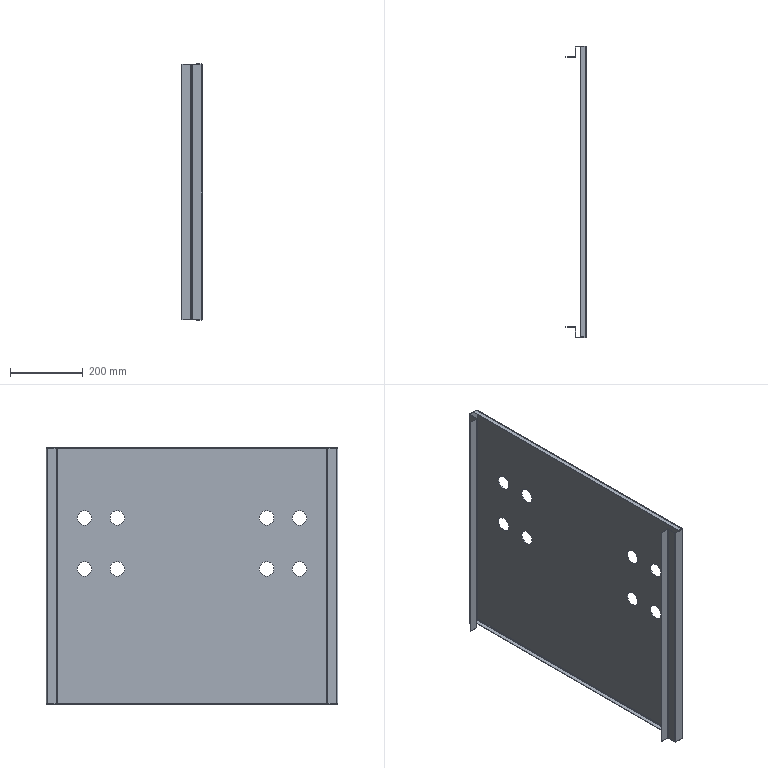Part | STEP file | YBQDJ-BJ-3 | 1 solid | 78 faces | box 55 x 800 x 705 mm | volume 823970 mm3 | plane 38 | cylinder 24 | spline 16 | commonest cylinder face diameters 3 x8 5.4 x8 40 x8